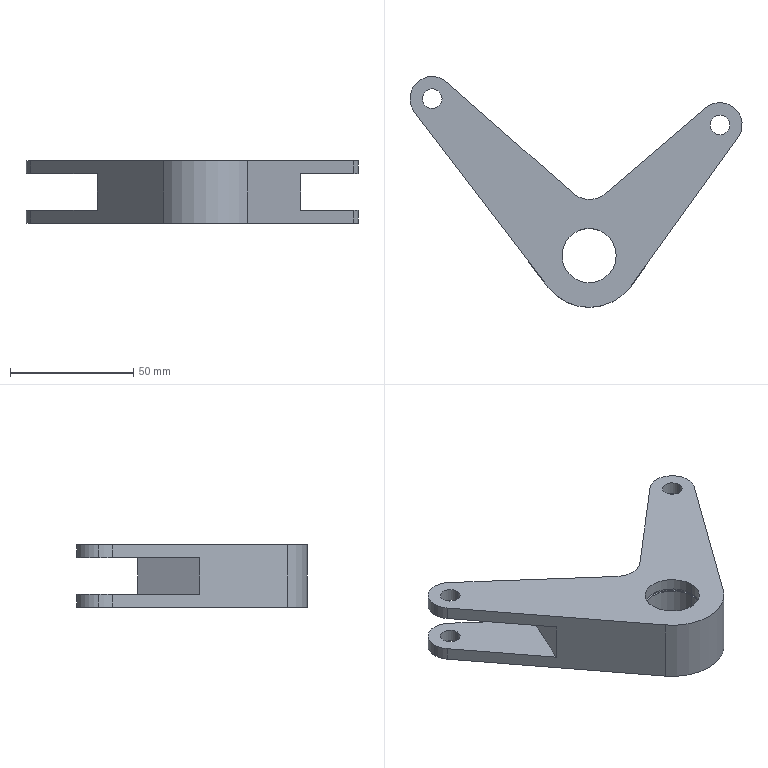Part | SolidWorks | features ICE 6, Extrusion 1, Fillet 1 | 1 solid | 42 faces | box 134.673 x 93.64 x 25.4 mm | volume 86753 mm3 | cylinder 26 | plane 16 | commonest cylinder face diameters 8 x8 18 x6 22 x6 23.3 x4 20 x1 42 x1
STEP:
#1=CARTESIAN_POINT('',(-11.65,0.,-8.1));
#2=VERTEX_POINT('',#1);
#3=CARTESIAN_POINT('',(11.65,0.,-8.1));
#4=VERTEX_POINT('',#3);
#5=CARTESIAN_POINT('',(0.,0.,-8.1));
#6=DIRECTION('',(0.,0.,1.));
#7=DIRECTION('',(1.,0.,0.));
#8=AXIS2_PLACEMENT_3D('',#5,#6,#7);
#9=CIRCLE('',#8,11.65);
#10=EDGE_CURVE('',#2,#4,#9,.T.);
#11=ORIENTED_EDGE('',*,*,#10,.F.);
#12=CARTESIAN_POINT('',(-11.65,0.,-7.));
#13=VERTEX_POINT('',#12);
#14=CARTESIAN_POINT('',(-11.65,0.,-8.1));
#15=DIRECTION('',(0.,0.,1.));
#16=VECTOR('',#15,1000.);
#17=LINE('',#14,#16);
#18=EDGE_CURVE('',#2,#13,#17,.T.);
#19=ORIENTED_EDGE('',*,*,#18,.T.);
#20=CARTESIAN_POINT('',(11.65,0.,-7.));
#21=VERTEX_POINT('',#20);
#22=CARTESIAN_POINT('',(0.,0.,-7.));
#23=DIRECTION('',(0.,0.,1.));
#24=DIRECTION('',(1.,0.,0.));
#25=AXIS2_PLACEMENT_3D('',#22,#23,#24);
#26=CIRCLE('',#25,11.65);
#27=EDGE_CURVE('',#13,#21,#26,.T.);
#28=ORIENTED_EDGE('',*,*,#27,.T.);
#29=CARTESIAN_POINT('',(11.65,0.,-8.1));
#30=DIRECTION('',(0.,0.,1.));
#31=VECTOR('',#30,1000.);
#32=LINE('',#29,#31);
#33=EDGE_CURVE('',#4,#21,#32,.T.);
#34=ORIENTED_EDGE('',*,*,#33,.F.);
#35=EDGE_LOOP('',(#11,#19,#28,#34));
#36=FACE_OUTER_BOUND('',#35,.T.);
#37=CARTESIAN_POINT('',(0.,0.,-8.1));
#38=DIRECTION('',(0.,0.,1.));
#39=DIRECTION('',(1.,0.,0.));
#40=AXIS2_PLACEMENT_3D('',#37,#38,#39);
#41=CYLINDRICAL_SURFACE('',#40,11.65);
#42=ADVANCED_FACE('',(#36),#41,.F.);
#43=CARTESIAN_POINT('',(-11.65,0.,8.1));
#44=VERTEX_POINT('',#43);
#45=CARTESIAN_POINT('',(11.65,0.,8.1));
#46=VERTEX_POINT('',#45);
#47=CARTESIAN_POINT('',(0.,0.,8.1));
#48=DIRECTION('',(0.,0.,1.));
#49=DIRECTION('',(1.,0.,0.));
#50=AXIS2_PLACEMENT_3D('',#47,#48,#49);
#51=CIRCLE('',#50,11.65);
#52=EDGE_CURVE('',#44,#46,#51,.T.);
#53=ORIENTED_EDGE('',*,*,#52,.T.);
#54=CARTESIAN_POINT('',(11.65,0.,7.));
#55=VERTEX_POINT('',#54);
#56=CARTESIAN_POINT('',(11.65,0.,8.1));
#57=DIRECTION('',(0.,0.,-1.));
#58=VECTOR('',#57,1000.);
#59=LINE('',#56,#58);
#60=EDGE_CURVE('',#46,#55,#59,.T.);
#61=ORIENTED_EDGE('',*,*,#60,.T.);
#62=CARTESIAN_POINT('',(-11.65,0.,7.));
#63=VERTEX_POINT('',#62);
#64=CARTESIAN_POINT('',(0.,0.,7.));
#65=DIRECTION('',(0.,0.,1.));
#66=DIRECTION('',(1.,0.,0.));
#67=AXIS2_PLACEMENT_3D('',#64,#65,#66);
#68=CIRCLE('',#67,11.65);
#69=EDGE_CURVE('',#63,#55,#68,.T.);
#70=ORIENTED_EDGE('',*,*,#69,.F.);
#71=CARTESIAN_POINT('',(-11.65,0.,8.1));
#72=DIRECTION('',(0.,0.,-1.));
#73=VECTOR('',#72,1000.);
#74=LINE('',#71,#73);
#75=EDGE_CURVE('',#44,#63,#74,.T.);
#76=ORIENTED_EDGE('',*,*,#75,.F.);
#77=EDGE_LOOP('',(#53,#61,#70,#76));
#78=FACE_OUTER_BOUND('',#77,.T.);
#79=CARTESIAN_POINT('',(0.,0.,8.1));
#80=DIRECTION('',(0.,0.,-1.));
#81=DIRECTION('',(-1.,0.,0.));
#82=AXIS2_PLACEMENT_3D('',#79,#80,#81);
#83=CYLINDRICAL_SURFACE('',#82,11.65);
#84=ADVANCED_FACE('',(#78),#83,.F.);
#85=CARTESIAN_POINT('',(-72.64,63.64,12.7));
#86=VERTEX_POINT('',#85);
#87=CARTESIAN_POINT('',(-70.795,58.181,12.7));
#88=VERTEX_POINT('',#87);
#89=CARTESIAN_POINT('',(-63.64,63.64,12.7));
#90=DIRECTION('',(0.,0.,1.));
#91=DIRECTION('',(1.,0.,0.));
#92=AXIS2_PLACEMENT_3D('',#89,#90,#91);
#93=CIRCLE('',#92,9.);
#94=EDGE_CURVE('',#86,#88,#93,.T.);
#95=ORIENTED_EDGE('',*,*,#94,.F.);
#96=CARTESIAN_POINT('',(-72.64,63.64,7.5));
#97=VERTEX_POINT('',#96);
#98=CARTESIAN_POINT('',(-72.64,63.64,12.7));
#99=DIRECTION('',(0.,0.,-1.));
#100=VECTOR('',#99,1000.);
#101=LINE('',#98,#100);
#102=EDGE_CURVE('',#86,#97,#101,.T.);
#103=ORIENTED_EDGE('',*,*,#102,.T.);
#104=CARTESIAN_POINT('',(-70.795,58.181,7.5));
#105=VERTEX_POINT('',#104);
#106=CARTESIAN_POINT('',(-63.64,63.64,7.5));
#107=DIRECTION('',(0.,0.,1.));
#108=DIRECTION('',(1.,0.,0.));
#109=AXIS2_PLACEMENT_3D('',#106,#107,#108);
#110=CIRCLE('',#109,9.);
#111=EDGE_CURVE('',#97,#105,#110,.T.);
#112=ORIENTED_EDGE('',*,*,#111,.T.);
#113=CARTESIAN_POINT('',(-70.795,58.181,12.7));
#114=DIRECTION('',(0.,0.,-1.));
#115=VECTOR('',#114,1000.);
#116=LINE('',#113,#115);
#117=EDGE_CURVE('',#88,#105,#116,.T.);
#118=ORIENTED_EDGE('',*,*,#117,.F.);
#119=EDGE_LOOP('',(#95,#103,#112,#118));
#120=FACE_OUTER_BOUND('',#119,.T.);
#121=CARTESIAN_POINT('',(-63.64,63.64,12.7));
#122=DIRECTION('',(0.,0.,-1.));
#123=DIRECTION('',(-1.,0.,0.));
#124=AXIS2_PLACEMENT_3D('',#121,#122,#123);
#125=CYLINDRICAL_SURFACE('',#124,9.);
#126=ADVANCED_FACE('',(#120),#125,.T.);
#127=CARTESIAN_POINT('',(49.033,53.033,12.7));
#128=VERTEX_POINT('',#127);
#129=CARTESIAN_POINT('',(57.033,53.033,12.7));
#130=VERTEX_POINT('',#129);
#131=CARTESIAN_POINT('',(53.033,53.033,12.7));
#132=DIRECTION('',(0.,0.,1.));
#133=DIRECTION('',(1.,0.,0.));
#134=AXIS2_PLACEMENT_3D('',#131,#132,#133);
#135=CIRCLE('',#134,4.);
#136=EDGE_CURVE('',#128,#130,#135,.T.);
#137=ORIENTED_EDGE('',*,*,#136,.T.);
#138=CARTESIAN_POINT('',(57.033,53.033,7.5));
#139=VERTEX_POINT('',#138);
#140=CARTESIAN_POINT('',(57.033,53.033,12.7));
#141=DIRECTION('',(0.,0.,-1.));
#142=VECTOR('',#141,1000.);
#143=LINE('',#140,#142);
#144=EDGE_CURVE('',#130,#139,#143,.T.);
#145=ORIENTED_EDGE('',*,*,#144,.T.);
#146=CARTESIAN_POINT('',(49.033,53.033,7.5));
#147=VERTEX_POINT('',#146);
#148=CARTESIAN_POINT('',(53.033,53.033,7.5));
#149=DIRECTION('',(0.,0.,1.));
#150=DIRECTION('',(1.,0.,0.));
#151=AXIS2_PLACEMENT_3D('',#148,#149,#150);
#152=CIRCLE('',#151,4.);
#153=EDGE_CURVE('',#147,#139,#152,.T.);
#154=ORIENTED_EDGE('',*,*,#153,.F.);
#155=CARTESIAN_POINT('',(49.033,53.033,12.7));
#156=DIRECTION('',(0.,0.,-1.));
#157=VECTOR('',#156,1000.);
#158=LINE('',#155,#157);
#159=EDGE_CURVE('',#128,#147,#158,.T.);
#160=ORIENTED_EDGE('',*,*,#159,.F.);
#161=EDGE_LOOP('',(#137,#145,#154,#160));
#162=FACE_OUTER_BOUND('',#161,.T.);
#163=CARTESIAN_POINT('',(53.033,53.033,12.7));
#164=DIRECTION('',(0.,0.,-1.));
#165=DIRECTION('',(-1.,0.,0.));
#166=AXIS2_PLACEMENT_3D('',#163,#164,#165);
#167=CYLINDRICAL_SURFACE('',#166,4.);
#168=ADVANCED_FACE('',(#162),#167,.F.);
#169=CARTESIAN_POINT('',(-67.64,63.64,12.7));
#170=VERTEX_POINT('',#169);
#171=CARTESIAN_POINT('',(-59.64,63.64,12.7));
#172=VERTEX_POINT('',#171);
#173=CARTESIAN_POINT('',(-63.64,63.64,12.7));
#174=DIRECTION('',(0.,0.,1.));
#175=DIRECTION('',(1.,0.,0.));
#176=AXIS2_PLACEMENT_3D('',#173,#174,#175);
#177=CIRCLE('',#176,4.);
#178=EDGE_CURVE('',#170,#172,#177,.T.);
#179=ORIENTED_EDGE('',*,*,#178,.T.);
#180=CARTESIAN_POINT('',(-59.64,63.64,7.5));
#181=VERTEX_POINT('',#180);
#182=CARTESIAN_POINT('',(-59.64,63.64,12.7));
#183=DIRECTION('',(0.,0.,-1.));
#184=VECTOR('',#183,1000.);
#185=LINE('',#182,#184);
#186=EDGE_CURVE('',#172,#181,#185,.T.);
#187=ORIENTED_EDGE('',*,*,#186,.T.);
#188=CARTESIAN_POINT('',(-67.64,63.64,7.5));
#189=VERTEX_POINT('',#188);
#190=CARTESIAN_POINT('',(-63.64,63.64,7.5));
#191=DIRECTION('',(0.,0.,1.));
#192=DIRECTION('',(1.,0.,0.));
#193=AXIS2_PLACEMENT_3D('',#190,#191,#192);
#194=CIRCLE('',#193,4.);
#195=EDGE_CURVE('',#189,#181,#194,.T.);
#196=ORIENTED_EDGE('',*,*,#195,.F.);
#197=CARTESIAN_POINT('',(-67.64,63.64,12.7));
#198=DIRECTION('',(0.,0.,-1.));
#199=VECTOR('',#198,1000.);
#200=LINE('',#197,#199);
#201=EDGE_CURVE('',#170,#189,#200,.T.);
#202=ORIENTED_EDGE('',*,*,#201,.F.);
#203=EDGE_LOOP('',(#179,#187,#196,#202));
#204=FACE_OUTER_BOUND('',#203,.T.);
#205=CARTESIAN_POINT('',(-63.64,63.64,12.7));
#206=DIRECTION('',(0.,0.,-1.));
#207=DIRECTION('',(-1.,0.,0.));
#208=AXIS2_PLACEMENT_3D('',#205,#206,#207);
#209=CYLINDRICAL_SURFACE('',#208,4.);
#210=ADVANCED_FACE('',(#204),#209,.F.);
#211=CARTESIAN_POINT('',(-11.,0.,12.7));
#212=VERTEX_POINT('',#211);
#213=CARTESIAN_POINT('',(11.,0.,12.7));
#214=VERTEX_POINT('',#213);
#215=CARTESIAN_POINT('',(0.,0.,12.7));
#216=DIRECTION('',(0.,0.,1.));
#217=DIRECTION('',(1.,0.,0.));
#218=AXIS2_PLACEMENT_3D('',#215,#216,#217);
#219=CIRCLE('',#218,11.);
#220=EDGE_CURVE('',#212,#214,#219,.T.);
#221=ORIENTED_EDGE('',*,*,#220,.T.);
#222=CARTESIAN_POINT('',(11.,0.,8.1));
#223=VERTEX_POINT('',#222);
#224=CARTESIAN_POINT('',(11.,0.,12.7));
#225=DIRECTION('',(0.,0.,-1.));
#226=VECTOR('',#225,1000.);
#227=LINE('',#224,#226);
#228=EDGE_CURVE('',#214,#223,#227,.T.);
#229=ORIENTED_EDGE('',*,*,#228,.T.);
#230=CARTESIAN_POINT('',(-11.,0.,8.1));
#231=VERTEX_POINT('',#230);
#232=CARTESIAN_POINT('',(0.,0.,8.1));
#233=DIRECTION('',(0.,0.,1.));
#234=DIRECTION('',(1.,0.,0.));
#235=AXIS2_PLACEMENT_3D('',#232,#233,#234);
#236=CIRCLE('',#235,11.);
#237=EDGE_CURVE('',#231,#223,#236,.T.);
#238=ORIENTED_EDGE('',*,*,#237,.F.);
#239=CARTESIAN_POINT('',(-11.,0.,12.7));
#240=DIRECTION('',(0.,0.,-1.));
#241=VECTOR('',#240,1000.);
#242=LINE('',#239,#241);
#243=EDGE_CURVE('',#212,#231,#242,.T.);
#244=ORIENTED_EDGE('',*,*,#243,.F.);
#245=EDGE_LOOP('',(#221,#229,#238,#244));
#246=FACE_OUTER_BOUND('',#245,.T.);
#247=CARTESIAN_POINT('',(0.,0.,12.7));
#248=DIRECTION('',(0.,0.,-1.));
#249=DIRECTION('',(-1.,0.,0.));
#250=AXIS2_PLACEMENT_3D('',#247,#248,#249);
#251=CYLINDRICAL_SURFACE('',#250,11.);
#252=ADVANCED_FACE('',(#246),#251,.F.);
#253=CARTESIAN_POINT('',(49.033,53.033,-7.5));
#254=VERTEX_POINT('',#253);
#255=CARTESIAN_POINT('',(57.033,53.033,-7.5));
#256=VERTEX_POINT('',#255);
#257=CARTESIAN_POINT('',(53.033,53.033,-7.5));
#258=DIRECTION('',(0.,0.,1.));
#259=DIRECTION('',(1.,0.,0.));
#260=AXIS2_PLACEMENT_3D('',#257,#258,#259);
#261=CIRCLE('',#260,4.);
#262=EDGE_CURVE('',#254,#256,#261,.T.);
#263=ORIENTED_EDGE('',*,*,#262,.T.);
#264=CARTESIAN_POINT('',(57.033,53.033,-12.7));
#265=VERTEX_POINT('',#264);
#266=CARTESIAN_POINT('',(57.033,53.033,12.7));
#267=DIRECTION('',(0.,0.,-1.));
#268=VECTOR('',#267,1000.);
#269=LINE('',#266,#268);
#270=EDGE_CURVE('',#256,#265,#269,.T.);
#271=ORIENTED_EDGE('',*,*,#270,.T.);
#272=CARTESIAN_POINT('',(49.033,53.033,-12.7));
#273=VERTEX_POINT('',#272);
#274=CARTESIAN_POINT('',(53.033,53.033,-12.7));
#275=DIRECTION('',(0.,0.,1.));
#276=DIRECTION('',(1.,0.,0.));
#277=AXIS2_PLACEMENT_3D('',#274,#275,#276);
#278=CIRCLE('',#277,4.);
#279=EDGE_CURVE('',#273,#265,#278,.T.);
#280=ORIENTED_EDGE('',*,*,#279,.F.);
#281=CARTESIAN_POINT('',(49.033,53.033,12.7));
#282=DIRECTION('',(0.,0.,-1.));
#283=VECTOR('',#282,1000.);
#284=LINE('',#281,#283);
#285=EDGE_CURVE('',#254,#273,#284,.T.);
#286=ORIENTED_EDGE('',*,*,#285,.F.);
#287=EDGE_LOOP('',(#263,#271,#280,#286));
#288=FACE_OUTER_BOUND('',#287,.T.);
#289=CARTESIAN_POINT('',(53.033,53.033,12.7));
#290=DIRECTION('',(0.,0.,-1.));
#291=DIRECTION('',(-1.,0.,0.));
#292=AXIS2_PLACEMENT_3D('',#289,#290,#291);
#293=CYLINDRICAL_SURFACE('',#292,4.);
#294=ADVANCED_FACE('',(#288),#293,.F.);
#295=CARTESIAN_POINT('',(-67.64,63.64,-7.5));
#296=VERTEX_POINT('',#295);
#297=CARTESIAN_POINT('',(-59.64,63.64,-7.5));
#298=VERTEX_POINT('',#297);
#299=CARTESIAN_POINT('',(-63.64,63.64,-7.5));
#300=DIRECTION('',(0.,0.,1.));
#301=DIRECTION('',(1.,0.,0.));
#302=AXIS2_PLACEMENT_3D('',#299,#300,#301);
#303=CIRCLE('',#302,4.);
#304=EDGE_CURVE('',#296,#298,#303,.T.);
#305=ORIENTED_EDGE('',*,*,#304,.T.);
#306=CARTESIAN_POINT('',(-59.64,63.64,-12.7));
#307=VERTEX_POINT('',#306);
#308=CARTESIAN_POINT('',(-59.64,63.64,12.7));
#309=DIRECTION('',(0.,0.,-1.));
#310=VECTOR('',#309,1000.);
#311=LINE('',#308,#310);
#312=EDGE_CURVE('',#298,#307,#311,.T.);
#313=ORIENTED_EDGE('',*,*,#312,.T.);
#314=CARTESIAN_POINT('',(-67.64,63.64,-12.7));
#315=VERTEX_POINT('',#314);
#316=CARTESIAN_POINT('',(-63.64,63.64,-12.7));
#317=DIRECTION('',(0.,0.,1.));
#318=DIRECTION('',(1.,0.,0.));
#319=AXIS2_PLACEMENT_3D('',#316,#317,#318);
#320=CIRCLE('',#319,4.);
#321=EDGE_CURVE('',#315,#307,#320,.T.);
#322=ORIENTED_EDGE('',*,*,#321,.F.);
#323=CARTESIAN_POINT('',(-67.64,63.64,12.7));
#324=DIRECTION('',(0.,0.,-1.));
#325=VECTOR('',#324,1000.);
#326=LINE('',#323,#325);
#327=EDGE_CURVE('',#296,#315,#326,.T.);
#328=ORIENTED_EDGE('',*,*,#327,.F.);
#329=EDGE_LOOP('',(#305,#313,#322,#328));
#330=FACE_OUTER_BOUND('',#329,.T.);
#331=CARTESIAN_POINT('',(-63.64,63.64,12.7));
#332=DIRECTION('',(0.,0.,-1.));
#333=DIRECTION('',(-1.,0.,0.));
#334=AXIS2_PLACEMENT_3D('',#331,#332,#333);
#335=CYLINDRICAL_SURFACE('',#334,4.);
#336=ADVANCED_FACE('',(#330),#335,.F.);
#337=CARTESIAN_POINT('',(-72.64,63.64,-7.5));
#338=VERTEX_POINT('',#337);
#339=CARTESIAN_POINT('',(-70.795,58.181,-7.5));
#340=VERTEX_POINT('',#339);
#341=CARTESIAN_POINT('',(-63.64,63.64,-7.5));
#342=DIRECTION('',(0.,0.,1.));
#343=DIRECTION('',(1.,0.,0.));
#344=AXIS2_PLACEMENT_3D('',#341,#342,#343);
#345=CIRCLE('',#344,9.);
#346=EDGE_CURVE('',#338,#340,#345,.T.);
#347=ORIENTED_EDGE('',*,*,#346,.F.);
#348=CARTESIAN_POINT('',(-72.64,63.64,-12.7));
#349=VERTEX_POINT('',#348);
#350=CARTESIAN_POINT('',(-72.64,63.64,12.7));
#351=DIRECTION('',(0.,0.,-1.));
#352=VECTOR('',#351,1000.);
#353=LINE('',#350,#352);
#354=EDGE_CURVE('',#338,#349,#353,.T.);
#355=ORIENTED_EDGE('',*,*,#354,.T.);
#356=CARTESIAN_POINT('',(-70.795,58.181,-12.7));
#357=VERTEX_POINT('',#356);
#358=CARTESIAN_POINT('',(-63.64,63.64,-12.7));
#359=DIRECTION('',(0.,0.,1.));
#360=DIRECTION('',(1.,0.,0.));
#361=AXIS2_PLACEMENT_3D('',#358,#359,#360);
#362=CIRCLE('',#361,9.);
#363=EDGE_CURVE('',#349,#357,#362,.T.);
#364=ORIENTED_EDGE('',*,*,#363,.T.);
#365=CARTESIAN_POINT('',(-70.795,58.181,12.7));
#366=DIRECTION('',(0.,0.,-1.));
#367=VECTOR('',#366,1000.);
#368=LINE('',#365,#367);
#369=EDGE_CURVE('',#340,#357,#368,.T.);
#370=ORIENTED_EDGE('',*,*,#369,.F.);
#371=EDGE_LOOP('',(#347,#355,#364,#370));
#372=FACE_OUTER_BOUND('',#371,.T.);
#373=CARTESIAN_POINT('',(-63.64,63.64,12.7));
#374=DIRECTION('',(0.,0.,-1.));
#375=DIRECTION('',(-1.,0.,0.));
#376=AXIS2_PLACEMENT_3D('',#373,#374,#375);
#377=CYLINDRICAL_SURFACE('',#376,9.);
#378=ADVANCED_FACE('',(#372),#377,.T.);
#379=CARTESIAN_POINT('',(-11.,0.,7.));
#380=VERTEX_POINT('',#379);
#381=CARTESIAN_POINT('',(11.,0.,7.));
#382=VERTEX_POINT('',#381);
#383=CARTESIAN_POINT('',(0.,0.,7.));
#384=DIRECTION('',(0.,0.,1.));
#385=DIRECTION('',(1.,0.,0.));
#386=AXIS2_PLACEMENT_3D('',#383,#384,#385);
#387=CIRCLE('',#386,11.);
#388=EDGE_CURVE('',#380,#382,#387,.T.);
#389=ORIENTED_EDGE('',*,*,#388,.T.);
#390=CARTESIAN_POINT('',(11.,0.,-7.));
#391=VERTEX_POINT('',#390);
#392=CARTESIAN_POINT('',(11.,0.,12.7));
#393=DIRECTION('',(0.,0.,-1.));
#394=VECTOR('',#393,1000.);
#395=LINE('',#392,#394);
#396=EDGE_CURVE('',#382,#391,#395,.T.);
#397=ORIENTED_EDGE('',*,*,#396,.T.);
#398=CARTESIAN_POINT('',(-11.,0.,-7.));
#399=VERTEX_POINT('',#398);
#400=CARTESIAN_POINT('',(0.,0.,-7.));
#401=DIRECTION('',(0.,0.,1.));
#402=DIRECTION('',(1.,0.,0.));
#403=AXIS2_PLACEMENT_3D('',#400,#401,#402);
#404=CIRCLE('',#403,11.);
#405=EDGE_CURVE('',#399,#391,#404,.T.);
#406=ORIENTED_EDGE('',*,*,#405,.F.);
#407=CARTESIAN_POINT('',(-11.,0.,12.7));
#408=DIRECTION('',(0.,0.,-1.));
#409=VECTOR('',#408,1000.);
#410=LINE('',#407,#409);
#411=EDGE_CURVE('',#380,#399,#410,.T.);
#412=ORIENTED_EDGE('',*,*,#411,.F.);
#413=EDGE_LOOP('',(#389,#397,#406,#412));
#414=FACE_OUTER_BOUND('',#413,.T.);
#415=CARTESIAN_POINT('',(0.,0.,12.7));
#416=DIRECTION('',(0.,0.,-1.));
#417=DIRECTION('',(-1.,0.,0.));
#418=AXIS2_PLACEMENT_3D('',#415,#416,#417);
#419=CYLINDRICAL_SURFACE('',#418,11.);
#420=ADVANCED_FACE('',(#414),#419,.F.);
#421=CARTESIAN_POINT('',(-11.,0.,-8.1));
#422=VERTEX_POINT('',#421);
#423=CARTESIAN_POINT('',(11.,0.,-8.1));
#424=VERTEX_POINT('',#423);
#425=CARTESIAN_POINT('',(0.,0.,-8.1));
#426=DIRECTION('',(0.,0.,1.));
#427=DIRECTION('',(1.,0.,0.));
#428=AXIS2_PLACEMENT_3D('',#425,#426,#427);
#429=CIRCLE('',#428,11.);
#430=EDGE_CURVE('',#422,#424,#429,.T.);
#431=ORIENTED_EDGE('',*,*,#430,.T.);
#432=CARTESIAN_POINT('',(11.,0.,-12.7));
#433=VERTEX_POINT('',#432);
#434=CARTESIAN_POINT('',(11.,0.,12.7));
#435=DIRECTION('',(0.,0.,-1.));
#436=VECTOR('',#435,1000.);
#437=LINE('',#434,#436);
#438=EDGE_CURVE('',#424,#433,#437,.T.);
#439=ORIENTED_EDGE('',*,*,#438,.T.);
#440=CARTESIAN_POINT('',(-11.,0.,-12.7));
#441=VERTEX_POINT('',#440);
#442=CARTESIAN_POINT('',(0.,0.,-12.7));
#443=DIRECTION('',(0.,0.,1.));
#444=DIRECTION('',(1.,0.,0.));
#445=AXIS2_PLACEMENT_3D('',#442,#443,#444);
#446=CIRCLE('',#445,11.);
#447=EDGE_CURVE('',#441,#433,#446,.T.);
#448=ORIENTED_EDGE('',*,*,#447,.F.);
#449=CARTESIAN_POINT('',(-11.,0.,12.7));
#450=DIRECTION('',(0.,0.,-1.));
#451=VECTOR('',#450,1000.);
#452=LINE('',#449,#451);
#453=EDGE_CURVE('',#422,#441,#452,.T.);
#454=ORIENTED_EDGE('',*,*,#453,.F.);
#455=EDGE_LOOP('',(#431,#439,#448,#454));
#456=FACE_OUTER_BOUND('',#455,.T.);
#457=CARTESIAN_POINT('',(0.,0.,12.7));
#458=DIRECTION('',(0.,0.,-1.));
#459=DIRECTION('',(-1.,0.,0.));
#460=AXIS2_PLACEMENT_3D('',#457,#458,#459);
#461=CYLINDRICAL_SURFACE('',#460,11.);
#462=ADVANCED_FACE('',(#456),#461,.F.);
#463=ORIENTED_EDGE('',*,*,#153,.T.);
#464=CARTESIAN_POINT('',(53.033,53.033,7.5));
#465=DIRECTION('',(0.,0.,1.));
#466=DIRECTION('',(1.,0.,0.));
#467=AXIS2_PLACEMENT_3D('',#464,#465,#466);
#468=CIRCLE('',#467,4.);
#469=EDGE_CURVE('',#139,#147,#468,.T.);
#470=ORIENTED_EDGE('',*,*,#469,.T.);
#471=EDGE_LOOP('',(#463,#470));
#472=FACE_BOUND('',#471,.T.);
#473=CARTESIAN_POINT('',(26.892,42.51,7.5));
#474=VERTEX_POINT('',#473);
#475=CARTESIAN_POINT('',(38.684,17.744,7.5));
#476=VERTEX_POINT('',#475);
#477=CARTESIAN_POINT('',(27.638,40.942,7.5));
#478=DIRECTION('',(0.4299,-0.9029,0.));
#479=VECTOR('',#478,1000.);
#480=LINE('',#477,#479);
#481=EDGE_CURVE('',#474,#476,#480,.T.);
#482=ORIENTED_EDGE('',*,*,#481,.F.);
#483=CARTESIAN_POINT('',(47.182,59.871,7.5));
#484=VERTEX_POINT('',#483);
#485=CARTESIAN_POINT('',(47.182,59.871,7.5));
#486=DIRECTION('',(-0.7598,-0.6501,0.));
#487=VECTOR('',#486,1000.);
#488=LINE('',#485,#487);
#489=EDGE_CURVE('',#484,#474,#488,.T.);
#490=ORIENTED_EDGE('',*,*,#489,.F.);
#491=CARTESIAN_POINT('',(60.333,47.769,7.5));
#492=VERTEX_POINT('',#491);
#493=CARTESIAN_POINT('',(53.033,53.033,7.5));
#494=DIRECTION('',(0.,0.,1.));
#495=DIRECTION('',(1.,0.,0.));
#496=AXIS2_PLACEMENT_3D('',#493,#494,#495);
#497=CIRCLE('',#496,9.);
#498=EDGE_CURVE('',#492,#484,#497,.T.);
#499=ORIENTED_EDGE('',*,*,#498,.F.);
#500=CARTESIAN_POINT('',(17.034,-12.282,7.5));
#501=DIRECTION('',(0.5849,0.8111,0.));
#502=VECTOR('',#501,1000.);
#503=LINE('',#500,#502);
#504=EDGE_CURVE('',#476,#492,#503,.T.);
#505=ORIENTED_EDGE('',*,*,#504,.F.);
#506=EDGE_LOOP('',(#482,#490,#499,#505));
#507=FACE_OUTER_BOUND('',#506,.T.);
#508=CARTESIAN_POINT('',(53.033,53.033,7.5));
#509=DIRECTION('',(0.,0.,1.));
#510=DIRECTION('',(1.,0.,0.));
#511=AXIS2_PLACEMENT_3D('',#508,#509,#510);
#512=PLANE('',#511);
#513=ADVANCED_FACE('',(#472,#507),#512,.F.);
#514=ORIENTED_EDGE('',*,*,#304,.F.);
#515=CARTESIAN_POINT('',(-63.64,63.64,-7.5));
#516=DIRECTION('',(0.,0.,1.));
#517=DIRECTION('',(1.,0.,0.));
#518=AXIS2_PLACEMENT_3D('',#515,#516,#517);
#519=CIRCLE('',#518,4.);
#520=EDGE_CURVE('',#298,#296,#519,.T.);
#521=ORIENTED_EDGE('',*,*,#520,.F.);
#522=EDGE_LOOP('',(#514,#521));
#523=FACE_BOUND('',#522,.T.);
#524=CARTESIAN_POINT('',(-43.746,22.722,-7.5));
#525=VERTEX_POINT('',#524);
#526=CARTESIAN_POINT('',(-70.795,58.181,-7.5));
#527=DIRECTION('',(0.6065,-0.7951,0.));
#528=VECTOR('',#527,1000.);
#529=LINE('',#526,#528);
#530=EDGE_CURVE('',#340,#525,#529,.T.);
#531=ORIENTED_EDGE('',*,*,#530,.T.);
#532=CARTESIAN_POINT('',(-32.101,47.818,-7.5));
#533=VERTEX_POINT('',#532);
#534=CARTESIAN_POINT('',(-15.026,84.614,-7.5));
#535=DIRECTION('',(0.4209,0.9071,0.));
#536=VECTOR('',#535,1000.);
#537=LINE('',#534,#536);
#538=EDGE_CURVE('',#525,#533,#537,.T.);
#539=ORIENTED_EDGE('',*,*,#538,.T.);
#540=CARTESIAN_POINT('',(-57.686,70.389,-7.5));
#541=VERTEX_POINT('',#540);
#542=CARTESIAN_POINT('',(-6.515,25.248,-7.5));
#543=DIRECTION('',(-0.7499,0.6615,0.));
#544=VECTOR('',#543,1000.);
#545=LINE('',#542,#544);
#546=EDGE_CURVE('',#533,#541,#545,.T.);
#547=ORIENTED_EDGE('',*,*,#546,.T.);
#548=CARTESIAN_POINT('',(-63.64,63.64,-7.5));
#549=DIRECTION('',(0.,0.,1.));
#550=DIRECTION('',(1.,0.,0.));
#551=AXIS2_PLACEMENT_3D('',#548,#549,#550);
#552=CIRCLE('',#551,9.);
#553=EDGE_CURVE('',#541,#338,#552,.T.);
#554=ORIENTED_EDGE('',*,*,#553,.T.);
#555=ORIENTED_EDGE('',*,*,#346,.T.);
#556=EDGE_LOOP('',(#531,#539,#547,#554,#555));
#557=FACE_OUTER_BOUND('',#556,.T.);
#558=CARTESIAN_POINT('',(53.033,53.033,-7.5));
#559=DIRECTION('',(0.,0.,1.));
#560=DIRECTION('',(1.,0.,0.));
#561=AXIS2_PLACEMENT_3D('',#558,#559,#560);
#562=PLANE('',#561);
#563=ADVANCED_FACE('',(#523,#557),#562,.T.);
#564=CARTESIAN_POINT('',(17.034,-12.282,12.7));
#565=VERTEX_POINT('',#564);
#566=CARTESIAN_POINT('',(17.034,-12.282,-12.7));
#567=VERTEX_POINT('',#566);
#568=CARTESIAN_POINT('',(17.034,-12.282,12.7));
#569=DIRECTION('',(0.,0.,-1.));
#570=VECTOR('',#569,1000.);
#571=LINE('',#568,#570);
#572=EDGE_CURVE('',#565,#567,#571,.T.);
#573=ORIENTED_EDGE('',*,*,#572,.F.);
#574=CARTESIAN_POINT('',(-16.697,-12.737,12.7));
#575=VERTEX_POINT('',#574);
#576=CARTESIAN_POINT('',(0.,0.,12.7));
#577=DIRECTION('',(0.,0.,1.));
#578=DIRECTION('',(1.,0.,0.));
#579=AXIS2_PLACEMENT_3D('',#576,#577,#578);
#580=CIRCLE('',#579,21.);
#581=EDGE_CURVE('',#575,#565,#580,.T.);
#582=ORIENTED_EDGE('',*,*,#581,.F.);
#583=CARTESIAN_POINT('',(-16.697,-12.737,-12.7));
#584=VERTEX_POINT('',#583);
#585=CARTESIAN_POINT('',(-16.697,-12.737,12.7));
#586=DIRECTION('',(0.,0.,-1.));
#587=VECTOR('',#586,1000.);
#588=LINE('',#585,#587);
#589=EDGE_CURVE('',#575,#584,#588,.T.);
#590=ORIENTED_EDGE('',*,*,#589,.T.);
#591=CARTESIAN_POINT('',(0.,0.,-12.7));
#592=DIRECTION('',(0.,0.,1.));
#593=DIRECTION('',(1.,0.,0.));
#594=AXIS2_PLACEMENT_3D('',#591,#592,#593);
#595=CIRCLE('',#594,21.);
#596=EDGE_CURVE('',#584,#567,#595,.T.);
#597=ORIENTED_EDGE('',*,*,#596,.T.);
#598=EDGE_LOOP('',(#573,#582,#590,#597));
#599=FACE_OUTER_BOUND('',#598,.T.);
#600=CARTESIAN_POINT('',(0.,0.,12.7));
#601=DIRECTION('',(0.,0.,-1.));
#602=DIRECTION('',(-1.,0.,0.));
#603=AXIS2_PLACEMENT_3D('',#600,#601,#602);
#604=CYLINDRICAL_SURFACE('',#603,21.);
#605=ADVANCED_FACE('',(#599),#604,.T.);
#606=ORIENTED_EDGE('',*,*,#262,.F.);
#607=CARTESIAN_POINT('',(53.033,53.033,-7.5));
#608=DIRECTION('',(0.,0.,1.));
#609=DIRECTION('',(1.,0.,0.));
#610=AXIS2_PLACEMENT_3D('',#607,#608,#609);
#611=CIRCLE('',#610,4.);
#612=EDGE_CURVE('',#256,#254,#611,.T.);
#613=ORIENTED_EDGE('',*,*,#612,.F.);
#614=EDGE_LOOP('',(#606,#613));
#615=FACE_BOUND('',#614,.T.);
#616=CARTESIAN_POINT('',(47.182,59.871,-7.5));
#617=VERTEX_POINT('',#616);
#618=CARTESIAN_POINT('',(26.892,42.51,-7.5));
#619=VERTEX_POINT('',#618);
#620=CARTESIAN_POINT('',(47.182,59.871,-7.5));
#621=DIRECTION('',(-0.7598,-0.6501,0.));
#622=VECTOR('',#621,1000.);
#623=LINE('',#620,#622);
#624=EDGE_CURVE('',#617,#619,#623,.T.);
#625=ORIENTED_EDGE('',*,*,#624,.T.);
#626=CARTESIAN_POINT('',(38.684,17.744,-7.5));
#627=VERTEX_POINT('',#626);
#628=CARTESIAN_POINT('',(27.638,40.942,-7.5));
#629=DIRECTION('',(0.4299,-0.9029,0.));
#630=VECTOR('',#629,1000.);
#631=LINE('',#628,#630);
#632=EDGE_CURVE('',#619,#627,#631,.T.);
#633=ORIENTED_EDGE('',*,*,#632,.T.);
#634=CARTESIAN_POINT('',(60.333,47.769,-7.5));
#635=VERTEX_POINT('',#634);
#636=CARTESIAN_POINT('',(17.034,-12.282,-7.5));
#637=DIRECTION('',(0.5849,0.8111,0.));
#638=VECTOR('',#637,1000.);
#639=LINE('',#636,#638);
#640=EDGE_CURVE('',#627,#635,#639,.T.);
#641=ORIENTED_EDGE('',*,*,#640,.T.);
#642=CARTESIAN_POINT('',(53.033,53.033,-7.5));
#643=DIRECTION('',(0.,0.,1.));
#644=DIRECTION('',(1.,0.,0.));
#645=AXIS2_PLACEMENT_3D('',#642,#643,#644);
#646=CIRCLE('',#645,9.);
#647=EDGE_CURVE('',#635,#617,#646,.T.);
#648=ORIENTED_EDGE('',*,*,#647,.T.);
#649=EDGE_LOOP('',(#625,#633,#641,#648));
#650=FACE_OUTER_BOUND('',#649,.T.);
#651=CARTESIAN_POINT('',(53.033,53.033,-7.5));
#652=DIRECTION('',(0.,0.,1.));
#653=DIRECTION('',(1.,0.,0.));
#654=AXIS2_PLACEMENT_3D('',#651,#652,#653);
#655=PLANE('',#654);
#656=ADVANCED_FACE('',(#615,#650),#655,.T.);
#657=ORIENTED_EDGE('',*,*,#195,.T.);
#658=CARTESIAN_POINT('',(-63.64,63.64,7.5));
#659=DIRECTION('',(0.,0.,1.));
#660=DIRECTION('',(1.,0.,0.));
#661=AXIS2_PLACEMENT_3D('',#658,#659,#660);
#662=CIRCLE('',#661,4.);
#663=EDGE_CURVE('',#181,#189,#662,.T.);
#664=ORIENTED_EDGE('',*,*,#663,.T.);
#665=EDGE_LOOP('',(#657,#664));
#666=FACE_BOUND('',#665,.T.);
#667=CARTESIAN_POINT('',(-43.746,22.722,7.5));
#668=VERTEX_POINT('',#667);
#669=CARTESIAN_POINT('',(-32.101,47.818,7.5));
#670=VERTEX_POINT('',#669);
#671=CARTESIAN_POINT('',(-15.026,84.614,7.5));
#672=DIRECTION('',(0.4209,0.9071,0.));
#673=VECTOR('',#672,1000.);
#674=LINE('',#671,#673);
#675=EDGE_CURVE('',#668,#670,#674,.T.);
#676=ORIENTED_EDGE('',*,*,#675,.F.);
#677=CARTESIAN_POINT('',(-70.795,58.181,7.5));
#678=DIRECTION('',(0.6065,-0.7951,0.));
#679=VECTOR('',#678,1000.);
#680=LINE('',#677,#679);
#681=EDGE_CURVE('',#105,#668,#680,.T.);
#682=ORIENTED_EDGE('',*,*,#681,.F.);
#683=ORIENTED_EDGE('',*,*,#111,.F.);
#684=CARTESIAN_POINT('',(-57.686,70.389,7.5));
#685=VERTEX_POINT('',#684);
#686=CARTESIAN_POINT('',(-63.64,63.64,7.5));
#687=DIRECTION('',(0.,0.,1.));
#688=DIRECTION('',(1.,0.,0.));
#689=AXIS2_PLACEMENT_3D('',#686,#687,#688);
#690=CIRCLE('',#689,9.);
#691=EDGE_CURVE('',#685,#97,#690,.T.);
#692=ORIENTED_EDGE('',*,*,#691,.F.);
#693=CARTESIAN_POINT('',(-6.515,25.248,7.5));
#694=DIRECTION('',(-0.7499,0.6615,0.));
#695=VECTOR('',#694,1000.);
#696=LINE('',#693,#695);
#697=EDGE_CURVE('',#670,#685,#696,.T.);
#698=ORIENTED_EDGE('',*,*,#697,.F.);
#699=EDGE_LOOP('',(#676,#682,#683,#692,#698));
#700=FACE_OUTER_BOUND('',#699,.T.);
#701=CARTESIAN_POINT('',(53.033,53.033,7.5));
#702=DIRECTION('',(0.,0.,1.));
#703=DIRECTION('',(1.,0.,0.));
#704=AXIS2_PLACEMENT_3D('',#701,#702,#703);
#705=PLANE('',#704);
#706=ADVANCED_FACE('',(#666,#700),#705,.F.);
#707=ORIENTED_EDGE('',*,*,#438,.F.);
#708=CARTESIAN_POINT('',(0.,0.,-8.1));
#709=DIRECTION('',(0.,0.,1.));
#710=DIRECTION('',(1.,0.,0.));
#711=AXIS2_PLACEMENT_3D('',#708,#709,#710);
#712=CIRCLE('',#711,11.);
#713=EDGE_CURVE('',#424,#422,#712,.T.);
#714=ORIENTED_EDGE('',*,*,#713,.T.);
#715=ORIENTED_EDGE('',*,*,#453,.T.);
#716=CARTESIAN_POINT('',(0.,0.,-12.7));
#717=DIRECTION('',(0.,0.,1.));
#718=DIRECTION('',(1.,0.,0.));
#719=AXIS2_PLACEMENT_3D('',#716,#717,#718);
#720=CIRCLE('',#719,11.);
#721=EDGE_CURVE('',#433,#441,#720,.T.);
#722=ORIENTED_EDGE('',*,*,#721,.F.);
#723=EDGE_LOOP('',(#707,#714,#715,#722));
#724=FACE_OUTER_BOUND('',#723,.T.);
#725=CARTESIAN_POINT('',(0.,0.,12.7));
#726=DIRECTION('',(0.,0.,-1.));
#727=DIRECTION('',(-1.,0.,0.));
#728=AXIS2_PLACEMENT_3D('',#725,#726,#727);
#729=CYLINDRICAL_SURFACE('',#728,11.);
#730=ADVANCED_FACE('',(#724),#729,.F.);
#731=ORIENTED_EDGE('',*,*,#396,.F.);
#732=CARTESIAN_POINT('',(0.,0.,7.));
#733=DIRECTION('',(0.,0.,1.));
#734=DIRECTION('',(1.,0.,0.));
#735=AXIS2_PLACEMENT_3D('',#732,#733,#734);
#736=CIRCLE('',#735,11.);
#737=EDGE_CURVE('',#382,#380,#736,.T.);
#738=ORIENTED_EDGE('',*,*,#737,.T.);
#739=ORIENTED_EDGE('',*,*,#411,.T.);
#740=CARTESIAN_POINT('',(0.,0.,-7.));
#741=DIRECTION('',(0.,0.,1.));
#742=DIRECTION('',(1.,0.,0.));
#743=AXIS2_PLACEMENT_3D('',#740,#741,#742);
#744=CIRCLE('',#743,11.);
#745=EDGE_CURVE('',#391,#399,#744,.T.);
#746=ORIENTED_EDGE('',*,*,#745,.F.);
#747=EDGE_LOOP('',(#731,#738,#739,#746));
#748=FACE_OUTER_BOUND('',#747,.T.);
#749=CARTESIAN_POINT('',(0.,0.,12.7));
#750=DIRECTION('',(0.,0.,-1.));
#751=DIRECTION('',(-1.,0.,0.));
#752=AXIS2_PLACEMENT_3D('',#749,#750,#751);
#753=CYLINDRICAL_SURFACE('',#752,11.);
#754=ADVANCED_FACE('',(#748),#753,.F.);
#755=ORIENTED_EDGE('',*,*,#354,.F.);
#756=ORIENTED_EDGE('',*,*,#553,.F.);
#757=CARTESIAN_POINT('',(-57.686,70.389,-12.7));
#758=VERTEX_POINT('',#757);
#759=CARTESIAN_POINT('',(-57.686,70.389,-12.7));
#760=DIRECTION('',(0.,0.,1.));
#761=VECTOR('',#760,1000.);
#762=LINE('',#759,#761);
#763=EDGE_CURVE('',#758,#541,#762,.T.);
#764=ORIENTED_EDGE('',*,*,#763,.F.);
#765=CARTESIAN_POINT('',(-63.64,63.64,-12.7));
#766=DIRECTION('',(0.,0.,1.));
#767=DIRECTION('',(1.,0.,0.));
#768=AXIS2_PLACEMENT_3D('',#765,#766,#767);
#769=CIRCLE('',#768,9.);
#770=EDGE_CURVE('',#758,#349,#769,.T.);
#771=ORIENTED_EDGE('',*,*,#770,.T.);
#772=EDGE_LOOP('',(#755,#756,#764,#771));
#773=FACE_OUTER_BOUND('',#772,.T.);
#774=CARTESIAN_POINT('',(-63.64,63.64,12.7));
#775=DIRECTION('',(0.,0.,-1.));
#776=DIRECTION('',(-1.,0.,0.));
#777=AXIS2_PLACEMENT_3D('',#774,#775,#776);
#778=CYLINDRICAL_SURFACE('',#777,9.);
#779=ADVANCED_FACE('',(#773),#778,.T.);
#780=CARTESIAN_POINT('',(-43.746,22.722,12.7));
#781=DIRECTION('',(0.,0.,-1.));
#782=VECTOR('',#781,1000.);
#783=LINE('',#780,#782);
#784=EDGE_CURVE('',#668,#525,#783,.T.);
#785=ORIENTED_EDGE('',*,*,#784,.T.);
#786=ORIENTED_EDGE('',*,*,#530,.F.);
#787=ORIENTED_EDGE('',*,*,#369,.T.);
#788=CARTESIAN_POINT('',(-16.697,-12.737,-12.7));
#789=DIRECTION('',(0.6065,-0.7951,0.));
#790=VECTOR('',#789,1000.);
#791=LINE('',#788,#790);
#792=EDGE_CURVE('',#357,#584,#791,.T.);
#793=ORIENTED_EDGE('',*,*,#792,.T.);
#794=ORIENTED_EDGE('',*,*,#589,.F.);
#795=CARTESIAN_POINT('',(-16.697,-12.737,12.7));
#796=DIRECTION('',(0.6065,-0.7951,0.));
#797=VECTOR('',#796,1000.);
#798=LINE('',#795,#797);
#799=EDGE_CURVE('',#88,#575,#798,.T.);
#800=ORIENTED_EDGE('',*,*,#799,.F.);
#801=ORIENTED_EDGE('',*,*,#117,.T.);
#802=ORIENTED_EDGE('',*,*,#681,.T.);
#803=EDGE_LOOP('',(#785,#786,#787,#793,#794,#800,#801,#802));
#804=FACE_OUTER_BOUND('',#803,.T.);
#805=CARTESIAN_POINT('',(-16.697,-12.737,12.7));
#806=DIRECTION('',(0.7951,0.6065,0.));
#807=DIRECTION('',(-0.6065,0.7951,0.));
#808=AXIS2_PLACEMENT_3D('',#805,#806,#807);
#809=PLANE('',#808);
#810=ADVANCED_FACE('',(#804),#809,.F.);
#811=CARTESIAN_POINT('',(38.684,17.744,12.7));
#812=DIRECTION('',(0.,0.,-1.));
#813=VECTOR('',#812,1000.);
#814=LINE('',#811,#813);
#815=EDGE_CURVE('',#476,#627,#814,.T.);
#816=ORIENTED_EDGE('',*,*,#815,.F.);
#817=ORIENTED_EDGE('',*,*,#504,.T.);
#818=CARTESIAN_POINT('',(60.333,47.769,12.7));
#819=VERTEX_POINT('',#818);
#820=CARTESIAN_POINT('',(60.333,47.769,12.7));
#821=DIRECTION('',(0.,0.,-1.));
#822=VECTOR('',#821,1000.);
#823=LINE('',#820,#822);
#824=EDGE_CURVE('',#819,#492,#823,.T.);
#825=ORIENTED_EDGE('',*,*,#824,.F.);
#826=CARTESIAN_POINT('',(17.034,-12.282,12.7));
#827=DIRECTION('',(0.5849,0.8111,0.));
#828=VECTOR('',#827,1000.);
#829=LINE('',#826,#828);
#830=EDGE_CURVE('',#565,#819,#829,.T.);
#831=ORIENTED_EDGE('',*,*,#830,.F.);
#832=ORIENTED_EDGE('',*,*,#572,.T.);
#833=CARTESIAN_POINT('',(60.333,47.769,-12.7));
#834=VERTEX_POINT('',#833);
#835=CARTESIAN_POINT('',(17.034,-12.282,-12.7));
#836=DIRECTION('',(0.5849,0.8111,0.));
#837=VECTOR('',#836,1000.);
#838=LINE('',#835,#837);
#839=EDGE_CURVE('',#567,#834,#838,.T.);
#840=ORIENTED_EDGE('',*,*,#839,.T.);
#841=CARTESIAN_POINT('',(60.333,47.769,12.7));
#842=DIRECTION('',(0.,0.,-1.));
#843=VECTOR('',#842,1000.);
#844=LINE('',#841,#843);
#845=EDGE_CURVE('',#635,#834,#844,.T.);
#846=ORIENTED_EDGE('',*,*,#845,.F.);
#847=ORIENTED_EDGE('',*,*,#640,.F.);
#848=EDGE_LOOP('',(#816,#817,#825,#831,#832,#840,#846,#847));
#849=FACE_OUTER_BOUND('',#848,.T.);
#850=CARTESIAN_POINT('',(17.034,-12.282,12.7));
#851=DIRECTION('',(-0.8111,0.5849,0.));
#852=DIRECTION('',(-0.5849,-0.8111,0.));
#853=AXIS2_PLACEMENT_3D('',#850,#851,#852);
#854=PLANE('',#853);
#855=ADVANCED_FACE('',(#849),#854,.F.);
#856=ORIENTED_EDGE('',*,*,#312,.F.);
#857=ORIENTED_EDGE('',*,*,#520,.T.);
#858=ORIENTED_EDGE('',*,*,#327,.T.);
#859=CARTESIAN_POINT('',(-63.64,63.64,-12.7));
#860=DIRECTION('',(0.,0.,1.));
#861=DIRECTION('',(1.,0.,0.));
#862=AXIS2_PLACEMENT_3D('',#859,#860,#861);
#863=CIRCLE('',#862,4.);
#864=EDGE_CURVE('',#307,#315,#863,.T.);
#865=ORIENTED_EDGE('',*,*,#864,.F.);
#866=EDGE_LOOP('',(#856,#857,#858,#865));
#867=FACE_OUTER_BOUND('',#866,.T.);
#868=CARTESIAN_POINT('',(-63.64,63.64,12.7));
#869=DIRECTION('',(0.,0.,-1.));
#870=DIRECTION('',(-1.,0.,0.));
#871=AXIS2_PLACEMENT_3D('',#868,#869,#870);
#872=CYLINDRICAL_SURFACE('',#871,4.);
#873=ADVANCED_FACE('',(#867),#872,.F.);
#874=ORIENTED_EDGE('',*,*,#270,.F.);
#875=ORIENTED_EDGE('',*,*,#612,.T.);
#876=ORIENTED_EDGE('',*,*,#285,.T.);
#877=CARTESIAN_POINT('',(53.033,53.033,-12.7));
#878=DIRECTION('',(0.,0.,1.));
#879=DIRECTION('',(1.,0.,0.));
#880=AXIS2_PLACEMENT_3D('',#877,#878,#879);
#881=CIRCLE('',#880,4.);
#882=EDGE_CURVE('',#265,#273,#881,.T.);
#883=ORIENTED_EDGE('',*,*,#882,.F.);
#884=EDGE_LOOP('',(#874,#875,#876,#883));
#885=FACE_OUTER_BOUND('',#884,.T.);
#886=CARTESIAN_POINT('',(53.033,53.033,12.7));
#887=DIRECTION('',(0.,0.,-1.));
#888=DIRECTION('',(-1.,0.,0.));
#889=AXIS2_PLACEMENT_3D('',#886,#887,#888);
#890=CYLINDRICAL_SURFACE('',#889,4.);
#891=ADVANCED_FACE('',(#885),#890,.F.);
#892=ORIENTED_EDGE('',*,*,#228,.F.);
#893=CARTESIAN_POINT('',(0.,0.,12.7));
#894=DIRECTION('',(0.,0.,1.));
#895=DIRECTION('',(1.,0.,0.));
#896=AXIS2_PLACEMENT_3D('',#893,#894,#895);
#897=CIRCLE('',#896,11.);
#898=EDGE_CURVE('',#214,#212,#897,.T.);
#899=ORIENTED_EDGE('',*,*,#898,.T.);
#900=ORIENTED_EDGE('',*,*,#243,.T.);
#901=CARTESIAN_POINT('',(0.,0.,8.1));
#902=DIRECTION('',(0.,0.,1.));
#903=DIRECTION('',(1.,0.,0.));
#904=AXIS2_PLACEMENT_3D('',#901,#902,#903);
#905=CIRCLE('',#904,11.);
#906=EDGE_CURVE('',#223,#231,#905,.T.);
#907=ORIENTED_EDGE('',*,*,#906,.F.);
#908=EDGE_LOOP('',(#892,#899,#900,#907));
#909=FACE_OUTER_BOUND('',#908,.T.);
#910=CARTESIAN_POINT('',(0.,0.,12.7));
#911=DIRECTION('',(0.,0.,-1.));
#912=DIRECTION('',(-1.,0.,0.));
#913=AXIS2_PLACEMENT_3D('',#910,#911,#912);
#914=CYLINDRICAL_SURFACE('',#913,11.);
#915=ADVANCED_FACE('',(#909),#914,.F.);
#916=ORIENTED_EDGE('',*,*,#647,.F.);
#917=ORIENTED_EDGE('',*,*,#845,.T.);
#918=CARTESIAN_POINT('',(47.182,59.871,-12.7));
#919=VERTEX_POINT('',#918);
#920=CARTESIAN_POINT('',(53.033,53.033,-12.7));
#921=DIRECTION('',(0.,0.,1.));
#922=DIRECTION('',(1.,0.,0.));
#923=AXIS2_PLACEMENT_3D('',#920,#921,#922);
#924=CIRCLE('',#923,9.);
#925=EDGE_CURVE('',#834,#919,#924,.T.);
#926=ORIENTED_EDGE('',*,*,#925,.T.);
#927=CARTESIAN_POINT('',(47.182,59.871,-12.7));
#928=DIRECTION('',(0.,0.,1.));
#929=VECTOR('',#928,1000.);
#930=LINE('',#927,#929);
#931=EDGE_CURVE('',#919,#617,#930,.T.);
#932=ORIENTED_EDGE('',*,*,#931,.T.);
#933=EDGE_LOOP('',(#916,#917,#926,#932));
#934=FACE_OUTER_BOUND('',#933,.T.);
#935=CARTESIAN_POINT('',(53.033,53.033,12.7));
#936=DIRECTION('',(0.,0.,-1.));
#937=DIRECTION('',(-1.,0.,0.));
#938=AXIS2_PLACEMENT_3D('',#935,#936,#937);
#939=CYLINDRICAL_SURFACE('',#938,9.);
#940=ADVANCED_FACE('',(#934),#939,.T.);
#941=CARTESIAN_POINT('',(6.601,25.149,-12.7));
#942=VERTEX_POINT('',#941);
#943=CARTESIAN_POINT('',(6.601,25.149,12.7));
#944=VERTEX_POINT('',#943);
#945=CARTESIAN_POINT('',(6.601,25.149,-12.7));
#946=DIRECTION('',(0.,0.,1.));
#947=VECTOR('',#946,1000.);
#948=LINE('',#945,#947);
#949=EDGE_CURVE('',#942,#944,#948,.T.);
#950=ORIENTED_EDGE('',*,*,#949,.T.);
#951=CARTESIAN_POINT('',(47.182,59.871,12.7));
#952=VERTEX_POINT('',#951);
#953=CARTESIAN_POINT('',(6.601,25.149,12.7));
#954=DIRECTION('',(0.7598,0.6501,0.));
#955=VECTOR('',#954,1000.);
#956=LINE('',#953,#955);
#957=EDGE_CURVE('',#944,#952,#956,.T.);
#958=ORIENTED_EDGE('',*,*,#957,.T.);
#959=CARTESIAN_POINT('',(47.182,59.871,-12.7));
#960=DIRECTION('',(0.,0.,1.));
#961=VECTOR('',#960,1000.);
#962=LINE('',#959,#961);
#963=EDGE_CURVE('',#484,#952,#962,.T.);
#964=ORIENTED_EDGE('',*,*,#963,.F.);
#965=ORIENTED_EDGE('',*,*,#489,.T.);
#966=CARTESIAN_POINT('',(26.892,42.51,12.7));
#967=DIRECTION('',(0.,0.,-1.));
#968=VECTOR('',#967,1000.);
#969=LINE('',#966,#968);
#970=EDGE_CURVE('',#474,#619,#969,.T.);
#971=ORIENTED_EDGE('',*,*,#970,.T.);
#972=ORIENTED_EDGE('',*,*,#624,.F.);
#973=ORIENTED_EDGE('',*,*,#931,.F.);
#974=CARTESIAN_POINT('',(6.601,25.149,-12.7));
#975=DIRECTION('',(0.7598,0.6501,0.));
#976=VECTOR('',#975,1000.);
#977=LINE('',#974,#976);
#978=EDGE_CURVE('',#942,#919,#977,.T.);
#979=ORIENTED_EDGE('',*,*,#978,.F.);
#980=EDGE_LOOP('',(#950,#958,#964,#965,#971,#972,#973,#979));
#981=FACE_OUTER_BOUND('',#980,.T.);
#982=CARTESIAN_POINT('',(6.601,25.149,-12.7));
#983=DIRECTION('',(0.6501,-0.7598,0.));
#984=DIRECTION('',(0.7598,0.6501,0.));
#985=AXIS2_PLACEMENT_3D('',#982,#983,#984);
#986=PLANE('',#985);
#987=ADVANCED_FACE('',(#981),#986,.F.);
#988=CARTESIAN_POINT('',(-6.515,25.248,-12.7));
#989=VERTEX_POINT('',#988);
#990=CARTESIAN_POINT('',(-6.515,25.248,12.7));
#991=VERTEX_POINT('',#990);
#992=CARTESIAN_POINT('',(-6.515,25.248,-12.7));
#993=DIRECTION('',(0.,0.,1.));
#994=VECTOR('',#993,1000.);
#995=LINE('',#992,#994);
#996=EDGE_CURVE('',#989,#991,#995,.T.);
#997=ORIENTED_EDGE('',*,*,#996,.T.);
#998=CARTESIAN_POINT('',(0.1001,32.747,12.7));
#999=DIRECTION('',(0.,0.,1.));
#1000=DIRECTION('',(1.,0.,0.));
#1001=AXIS2_PLACEMENT_3D('',#998,#999,#1000);
#1002=CIRCLE('',#1001,10.);
#1003=EDGE_CURVE('',#991,#944,#1002,.T.);
#1004=ORIENTED_EDGE('',*,*,#1003,.T.);
#1005=ORIENTED_EDGE('',*,*,#949,.F.);
#1006=CARTESIAN_POINT('',(0.1001,32.747,-12.7));
#1007=DIRECTION('',(0.,0.,1.));
#1008=DIRECTION('',(1.,0.,0.));
#1009=AXIS2_PLACEMENT_3D('',#1006,#1007,#1008);
#1010=CIRCLE('',#1009,10.);
#1011=EDGE_CURVE('',#989,#942,#1010,.T.);
#1012=ORIENTED_EDGE('',*,*,#1011,.F.);
#1013=EDGE_LOOP('',(#997,#1004,#1005,#1012));
#1014=FACE_OUTER_BOUND('',#1013,.T.);
#1015=CARTESIAN_POINT('',(0.1001,32.747,-12.7));
#1016=DIRECTION('',(0.,0.,1.));
#1017=DIRECTION('',(1.,0.,0.));
#1018=AXIS2_PLACEMENT_3D('',#1015,#1016,#1017);
#1019=CYLINDRICAL_SURFACE('',#1018,10.);
#1020=ADVANCED_FACE('',(#1014),#1019,.F.);
#1021=ORIENTED_EDGE('',*,*,#996,.F.);
#1022=CARTESIAN_POINT('',(-57.686,70.389,-12.7));
#1023=DIRECTION('',(0.7499,-0.6615,0.));
#1024=VECTOR('',#1023,1000.);
#1025=LINE('',#1022,#1024);
#1026=EDGE_CURVE('',#758,#989,#1025,.T.);
#1027=ORIENTED_EDGE('',*,*,#1026,.F.);
#1028=ORIENTED_EDGE('',*,*,#763,.T.);
#1029=ORIENTED_EDGE('',*,*,#546,.F.);
#1030=CARTESIAN_POINT('',(-32.101,47.818,12.7));
#1031=DIRECTION('',(0.,0.,-1.));
#1032=VECTOR('',#1031,1000.);
#1033=LINE('',#1030,#1032);
#1034=EDGE_CURVE('',#670,#533,#1033,.T.);
#1035=ORIENTED_EDGE('',*,*,#1034,.F.);
#1036=ORIENTED_EDGE('',*,*,#697,.T.);
#1037=CARTESIAN_POINT('',(-57.686,70.389,12.7));
#1038=VERTEX_POINT('',#1037);
#1039=CARTESIAN_POINT('',(-57.686,70.389,-12.7));
#1040=DIRECTION('',(0.,0.,1.));
#1041=VECTOR('',#1040,1000.);
#1042=LINE('',#1039,#1041);
#1043=EDGE_CURVE('',#685,#1038,#1042,.T.);
#1044=ORIENTED_EDGE('',*,*,#1043,.T.);
#1045=CARTESIAN_POINT('',(-57.686,70.389,12.7));
#1046=DIRECTION('',(0.7499,-0.6615,0.));
#1047=VECTOR('',#1046,1000.);
#1048=LINE('',#1045,#1047);
#1049=EDGE_CURVE('',#1038,#991,#1048,.T.);
#1050=ORIENTED_EDGE('',*,*,#1049,.T.);
#1051=EDGE_LOOP('',(#1021,#1027,#1028,#1029,#1035,#1036,#1044,#1050));
#1052=FACE_OUTER_BOUND('',#1051,.T.);
#1053=CARTESIAN_POINT('',(-57.686,70.389,-12.7));
#1054=DIRECTION('',(-0.6615,-0.7499,0.));
#1055=DIRECTION('',(0.7499,-0.6615,0.));
#1056=AXIS2_PLACEMENT_3D('',#1053,#1054,#1055);
#1057=PLANE('',#1056);
#1058=ADVANCED_FACE('',(#1052),#1057,.F.);
#1059=ORIENTED_EDGE('',*,*,#978,.T.);
#1060=ORIENTED_EDGE('',*,*,#925,.F.);
#1061=ORIENTED_EDGE('',*,*,#839,.F.);
#1062=ORIENTED_EDGE('',*,*,#596,.F.);
#1063=ORIENTED_EDGE('',*,*,#792,.F.);
#1064=ORIENTED_EDGE('',*,*,#363,.F.);
#1065=ORIENTED_EDGE('',*,*,#770,.F.);
#1066=ORIENTED_EDGE('',*,*,#1026,.T.);
#1067=ORIENTED_EDGE('',*,*,#1011,.T.);
#1068=EDGE_LOOP('',(#1059,#1060,#1061,#1062,#1063,#1064,#1065,#1066,#1067));
#1069=FACE_OUTER_BOUND('',#1068,.T.);
#1070=ORIENTED_EDGE('',*,*,#447,.T.);
#1071=ORIENTED_EDGE('',*,*,#721,.T.);
#1072=EDGE_LOOP('',(#1070,#1071));
#1073=FACE_BOUND('',#1072,.T.);
#1074=ORIENTED_EDGE('',*,*,#321,.T.);
#1075=ORIENTED_EDGE('',*,*,#864,.T.);
#1076=EDGE_LOOP('',(#1074,#1075));
#1077=FACE_BOUND('',#1076,.T.);
#1078=ORIENTED_EDGE('',*,*,#279,.T.);
#1079=ORIENTED_EDGE('',*,*,#882,.T.);
#1080=EDGE_LOOP('',(#1078,#1079));
#1081=FACE_BOUND('',#1080,.T.);
#1082=CARTESIAN_POINT('',(0.,0.,-12.7));
#1083=DIRECTION('',(0.,0.,1.));
#1084=DIRECTION('',(1.,0.,0.));
#1085=AXIS2_PLACEMENT_3D('',#1082,#1083,#1084);
#1086=PLANE('',#1085);
#1087=ADVANCED_FACE('',(#1069,#1073,#1077,#1081),#1086,.F.);
#1088=ORIENTED_EDGE('',*,*,#830,.T.);
#1089=CARTESIAN_POINT('',(53.033,53.033,12.7));
#1090=DIRECTION('',(0.,0.,1.));
#1091=DIRECTION('',(1.,0.,0.));
#1092=AXIS2_PLACEMENT_3D('',#1089,#1090,#1091);
#1093=CIRCLE('',#1092,9.);
#1094=EDGE_CURVE('',#819,#952,#1093,.T.);
#1095=ORIENTED_EDGE('',*,*,#1094,.T.);
#1096=ORIENTED_EDGE('',*,*,#957,.F.);
#1097=ORIENTED_EDGE('',*,*,#1003,.F.);
#1098=ORIENTED_EDGE('',*,*,#1049,.F.);
#1099=CARTESIAN_POINT('',(-63.64,63.64,12.7));
#1100=DIRECTION('',(0.,0.,1.));
#1101=DIRECTION('',(1.,0.,0.));
#1102=AXIS2_PLACEMENT_3D('',#1099,#1100,#1101);
#1103=CIRCLE('',#1102,9.);
#1104=EDGE_CURVE('',#1038,#86,#1103,.T.);
#1105=ORIENTED_EDGE('',*,*,#1104,.T.);
#1106=ORIENTED_EDGE('',*,*,#94,.T.);
#1107=ORIENTED_EDGE('',*,*,#799,.T.);
#1108=ORIENTED_EDGE('',*,*,#581,.T.);
#1109=EDGE_LOOP('',(#1088,#1095,#1096,#1097,#1098,#1105,#1106,#1107,#1108));
#1110=FACE_OUTER_BOUND('',#1109,.T.);
#1111=ORIENTED_EDGE('',*,*,#220,.F.);
#1112=ORIENTED_EDGE('',*,*,#898,.F.);
#1113=EDGE_LOOP('',(#1111,#1112));
#1114=FACE_BOUND('',#1113,.T.);
#1115=ORIENTED_EDGE('',*,*,#178,.F.);
#1116=CARTESIAN_POINT('',(-63.64,63.64,12.7));
#1117=DIRECTION('',(0.,0.,1.));
#1118=DIRECTION('',(1.,0.,0.));
#1119=AXIS2_PLACEMENT_3D('',#1116,#1117,#1118);
#1120=CIRCLE('',#1119,4.);
#1121=EDGE_CURVE('',#172,#170,#1120,.T.);
#1122=ORIENTED_EDGE('',*,*,#1121,.F.);
#1123=EDGE_LOOP('',(#1115,#1122));
#1124=FACE_BOUND('',#1123,.T.);
#1125=ORIENTED_EDGE('',*,*,#136,.F.);
#1126=CARTESIAN_POINT('',(53.033,53.033,12.7));
#1127=DIRECTION('',(0.,0.,1.));
#1128=DIRECTION('',(1.,0.,0.));
#1129=AXIS2_PLACEMENT_3D('',#1126,#1127,#1128);
#1130=CIRCLE('',#1129,4.);
#1131=EDGE_CURVE('',#130,#128,#1130,.T.);
#1132=ORIENTED_EDGE('',*,*,#1131,.F.);
#1133=EDGE_LOOP('',(#1125,#1132));
#1134=FACE_BOUND('',#1133,.T.);
#1135=CARTESIAN_POINT('',(0.,0.,12.7));
#1136=DIRECTION('',(0.,0.,1.));
#1137=DIRECTION('',(1.,0.,0.));
#1138=AXIS2_PLACEMENT_3D('',#1135,#1136,#1137);
#1139=PLANE('',#1138);
#1140=ADVANCED_FACE('',(#1110,#1114,#1124,#1134),#1139,.T.);
#1141=ORIENTED_EDGE('',*,*,#186,.F.);
#1142=ORIENTED_EDGE('',*,*,#1121,.T.);
#1143=ORIENTED_EDGE('',*,*,#201,.T.);
#1144=ORIENTED_EDGE('',*,*,#663,.F.);
#1145=EDGE_LOOP('',(#1141,#1142,#1143,#1144));
#1146=FACE_OUTER_BOUND('',#1145,.T.);
#1147=CARTESIAN_POINT('',(-63.64,63.64,12.7));
#1148=DIRECTION('',(0.,0.,-1.));
#1149=DIRECTION('',(-1.,0.,0.));
#1150=AXIS2_PLACEMENT_3D('',#1147,#1148,#1149);
#1151=CYLINDRICAL_SURFACE('',#1150,4.);
#1152=ADVANCED_FACE('',(#1146),#1151,.F.);
#1153=ORIENTED_EDGE('',*,*,#144,.F.);
#1154=ORIENTED_EDGE('',*,*,#1131,.T.);
#1155=ORIENTED_EDGE('',*,*,#159,.T.);
#1156=ORIENTED_EDGE('',*,*,#469,.F.);
#1157=EDGE_LOOP('',(#1153,#1154,#1155,#1156));
#1158=FACE_OUTER_BOUND('',#1157,.T.);
#1159=CARTESIAN_POINT('',(53.033,53.033,12.7));
#1160=DIRECTION('',(0.,0.,-1.));
#1161=DIRECTION('',(-1.,0.,0.));
#1162=AXIS2_PLACEMENT_3D('',#1159,#1160,#1161);
#1163=CYLINDRICAL_SURFACE('',#1162,4.);
#1164=ADVANCED_FACE('',(#1158),#1163,.F.);
#1165=ORIENTED_EDGE('',*,*,#824,.T.);
#1166=ORIENTED_EDGE('',*,*,#498,.T.);
#1167=ORIENTED_EDGE('',*,*,#963,.T.);
#1168=ORIENTED_EDGE('',*,*,#1094,.F.);
#1169=EDGE_LOOP('',(#1165,#1166,#1167,#1168));
#1170=FACE_OUTER_BOUND('',#1169,.T.);
#1171=CARTESIAN_POINT('',(53.033,53.033,12.7));
#1172=DIRECTION('',(0.,0.,-1.));
#1173=DIRECTION('',(-1.,0.,0.));
#1174=AXIS2_PLACEMENT_3D('',#1171,#1172,#1173);
#1175=CYLINDRICAL_SURFACE('',#1174,9.);
#1176=ADVANCED_FACE('',(#1170),#1175,.T.);
#1177=ORIENTED_EDGE('',*,*,#102,.F.);
#1178=ORIENTED_EDGE('',*,*,#1104,.F.);
#1179=ORIENTED_EDGE('',*,*,#1043,.F.);
#1180=ORIENTED_EDGE('',*,*,#691,.T.);
#1181=EDGE_LOOP('',(#1177,#1178,#1179,#1180));
#1182=FACE_OUTER_BOUND('',#1181,.T.);
#1183=CARTESIAN_POINT('',(-63.64,63.64,12.7));
#1184=DIRECTION('',(0.,0.,-1.));
#1185=DIRECTION('',(-1.,0.,0.));
#1186=AXIS2_PLACEMENT_3D('',#1183,#1184,#1185);
#1187=CYLINDRICAL_SURFACE('',#1186,9.);
#1188=ADVANCED_FACE('',(#1182),#1187,.T.);
#1189=ORIENTED_EDGE('',*,*,#60,.F.);
#1190=CARTESIAN_POINT('',(0.,0.,8.1));
#1191=DIRECTION('',(0.,0.,1.));
#1192=DIRECTION('',(1.,0.,0.));
#1193=AXIS2_PLACEMENT_3D('',#1190,#1191,#1192);
#1194=CIRCLE('',#1193,11.65);
#1195=EDGE_CURVE('',#46,#44,#1194,.T.);
#1196=ORIENTED_EDGE('',*,*,#1195,.T.);
#1197=ORIENTED_EDGE('',*,*,#75,.T.);
#1198=CARTESIAN_POINT('',(0.,0.,7.));
#1199=DIRECTION('',(0.,0.,1.));
#1200=DIRECTION('',(1.,0.,0.));
#1201=AXIS2_PLACEMENT_3D('',#1198,#1199,#1200);
#1202=CIRCLE('',#1201,11.65);
#1203=EDGE_CURVE('',#55,#63,#1202,.T.);
#1204=ORIENTED_EDGE('',*,*,#1203,.F.);
#1205=EDGE_LOOP('',(#1189,#1196,#1197,#1204));
#1206=FACE_OUTER_BOUND('',#1205,.T.);
#1207=CARTESIAN_POINT('',(0.,0.,8.1));
#1208=DIRECTION('',(0.,0.,-1.));
#1209=DIRECTION('',(-1.,0.,0.));
#1210=AXIS2_PLACEMENT_3D('',#1207,#1208,#1209);
#1211=CYLINDRICAL_SURFACE('',#1210,11.65);
#1212=ADVANCED_FACE('',(#1206),#1211,.F.);
#1213=ORIENTED_EDGE('',*,*,#237,.T.);
#1214=ORIENTED_EDGE('',*,*,#906,.T.);
#1215=EDGE_LOOP('',(#1213,#1214));
#1216=FACE_BOUND('',#1215,.T.);
#1217=ORIENTED_EDGE('',*,*,#52,.F.);
#1218=ORIENTED_EDGE('',*,*,#1195,.F.);
#1219=EDGE_LOOP('',(#1217,#1218));
#1220=FACE_OUTER_BOUND('',#1219,.T.);
#1221=CARTESIAN_POINT('',(0.,0.,8.1));
#1222=DIRECTION('',(0.,0.,1.));
#1223=DIRECTION('',(1.,0.,0.));
#1224=AXIS2_PLACEMENT_3D('',#1221,#1222,#1223);
#1225=PLANE('',#1224);
#1226=ADVANCED_FACE('',(#1216,#1220),#1225,.F.);
#1227=ORIENTED_EDGE('',*,*,#388,.F.);
#1228=ORIENTED_EDGE('',*,*,#737,.F.);
#1229=EDGE_LOOP('',(#1227,#1228));
#1230=FACE_BOUND('',#1229,.T.);
#1231=ORIENTED_EDGE('',*,*,#69,.T.);
#1232=ORIENTED_EDGE('',*,*,#1203,.T.);
#1233=EDGE_LOOP('',(#1231,#1232));
#1234=FACE_OUTER_BOUND('',#1233,.T.);
#1235=CARTESIAN_POINT('',(0.,0.,7.));
#1236=DIRECTION('',(0.,0.,1.));
#1237=DIRECTION('',(1.,0.,0.));
#1238=AXIS2_PLACEMENT_3D('',#1235,#1236,#1237);
#1239=PLANE('',#1238);
#1240=ADVANCED_FACE('',(#1230,#1234),#1239,.T.);
#1241=ORIENTED_EDGE('',*,*,#18,.F.);
#1242=CARTESIAN_POINT('',(0.,0.,-8.1));
#1243=DIRECTION('',(0.,0.,1.));
#1244=DIRECTION('',(1.,0.,0.));
#1245=AXIS2_PLACEMENT_3D('',#1242,#1243,#1244);
#1246=CIRCLE('',#1245,11.65);
#1247=EDGE_CURVE('',#4,#2,#1246,.T.);
#1248=ORIENTED_EDGE('',*,*,#1247,.F.);
#1249=ORIENTED_EDGE('',*,*,#33,.T.);
#1250=CARTESIAN_POINT('',(0.,0.,-7.));
#1251=DIRECTION('',(0.,0.,1.));
#1252=DIRECTION('',(1.,0.,0.));
#1253=AXIS2_PLACEMENT_3D('',#1250,#1251,#1252);
#1254=CIRCLE('',#1253,11.65);
#1255=EDGE_CURVE('',#21,#13,#1254,.T.);
#1256=ORIENTED_EDGE('',*,*,#1255,.T.);
#1257=EDGE_LOOP('',(#1241,#1248,#1249,#1256));
#1258=FACE_OUTER_BOUND('',#1257,.T.);
#1259=CARTESIAN_POINT('',(0.,0.,-8.1));
#1260=DIRECTION('',(0.,0.,1.));
#1261=DIRECTION('',(1.,0.,0.));
#1262=AXIS2_PLACEMENT_3D('',#1259,#1260,#1261);
#1263=CYLINDRICAL_SURFACE('',#1262,11.65);
#1264=ADVANCED_FACE('',(#1258),#1263,.F.);
#1265=ORIENTED_EDGE('',*,*,#430,.F.);
#1266=ORIENTED_EDGE('',*,*,#713,.F.);
#1267=EDGE_LOOP('',(#1265,#1266));
#1268=FACE_BOUND('',#1267,.T.);
#1269=ORIENTED_EDGE('',*,*,#1247,.T.);
#1270=ORIENTED_EDGE('',*,*,#10,.T.);
#1271=EDGE_LOOP('',(#1269,#1270));
#1272=FACE_OUTER_BOUND('',#1271,.T.);
#1273=CARTESIAN_POINT('',(0.,0.,-8.1));
#1274=DIRECTION('',(0.,0.,1.));
#1275=DIRECTION('',(1.,0.,0.));
#1276=AXIS2_PLACEMENT_3D('',#1273,#1274,#1275);
#1277=PLANE('',#1276);
#1278=ADVANCED_FACE('',(#1268,#1272),#1277,.T.);
#1279=ORIENTED_EDGE('',*,*,#405,.T.);
#1280=ORIENTED_EDGE('',*,*,#745,.T.);
#1281=EDGE_LOOP('',(#1279,#1280));
#1282=FACE_BOUND('',#1281,.T.);
#1283=ORIENTED_EDGE('',*,*,#1255,.F.);
#1284=ORIENTED_EDGE('',*,*,#27,.F.);
#1285=EDGE_LOOP('',(#1283,#1284));
#1286=FACE_OUTER_BOUND('',#1285,.T.);
#1287=CARTESIAN_POINT('',(0.,0.,-7.));
#1288=DIRECTION('',(0.,0.,1.));
#1289=DIRECTION('',(1.,0.,0.));
#1290=AXIS2_PLACEMENT_3D('',#1287,#1288,#1289);
#1291=PLANE('',#1290);
#1292=ADVANCED_FACE('',(#1282,#1286),#1291,.F.);
#1293=ORIENTED_EDGE('',*,*,#970,.F.);
#1294=ORIENTED_EDGE('',*,*,#481,.T.);
#1295=ORIENTED_EDGE('',*,*,#815,.T.);
#1296=ORIENTED_EDGE('',*,*,#632,.F.);
#1297=EDGE_LOOP('',(#1293,#1294,#1295,#1296));
#1298=FACE_OUTER_BOUND('',#1297,.T.);
#1299=CARTESIAN_POINT('',(38.684,17.744,12.7));
#1300=DIRECTION('',(-0.9029,-0.4299,0.));
#1301=DIRECTION('',(0.4299,-0.9029,0.));
#1302=AXIS2_PLACEMENT_3D('',#1299,#1300,#1301);
#1303=PLANE('',#1302);
#1304=ADVANCED_FACE('',(#1298),#1303,.F.);
#1305=ORIENTED_EDGE('',*,*,#538,.F.);
#1306=ORIENTED_EDGE('',*,*,#784,.F.);
#1307=ORIENTED_EDGE('',*,*,#675,.T.);
#1308=ORIENTED_EDGE('',*,*,#1034,.T.);
#1309=EDGE_LOOP('',(#1305,#1306,#1307,#1308));
#1310=FACE_OUTER_BOUND('',#1309,.T.);
#1311=CARTESIAN_POINT('',(-32.101,47.818,12.7));
#1312=DIRECTION('',(0.9071,-0.4209,0.));
#1313=DIRECTION('',(0.4209,0.9071,0.));
#1314=AXIS2_PLACEMENT_3D('',#1311,#1312,#1313);
#1315=PLANE('',#1314);
#1316=ADVANCED_FACE('',(#1310),#1315,.F.);
#1317=CLOSED_SHELL('',(#42,#84,#126,#168,#210,#252,#294,#336,#378,#420,#462,#513,#563,#605,#656,#706,#730,#754,#779,#810,#855,#873,#891,#915,#940,#987,#1020,#1058,#1087,#1140,#1152,#1164,#1176,#1188,#1212,#1226,#1240,#1264,#1278,#1292,#1304,#1316));
#1318=MANIFOLD_SOLID_BREP('',#1317);
#1319=CARTESIAN_POINT('',(0.,0.,0.));
#1320=DIRECTION('',(0.,0.,1.));
#1321=DIRECTION('',(1.,0.,0.));
#1322=AXIS2_PLACEMENT_3D('',#1319,#1320,#1321);
#1323=(LENGTH_UNIT()NAMED_UNIT(*)SI_UNIT(.MILLI.,.METRE.));
#1324=UNCERTAINTY_MEASURE_WITH_UNIT(LENGTH_MEASURE(0.00001),#1323,'','');
#1325=(NAMED_UNIT(*)PLANE_ANGLE_UNIT()SI_UNIT($,.RADIAN.));
#1326=(NAMED_UNIT(*)SI_UNIT($,.STERADIAN.)SOLID_ANGLE_UNIT());
#1327=(GEOMETRIC_REPRESENTATION_CONTEXT(3)GLOBAL_UNCERTAINTY_ASSIGNED_CONTEXT((#1324))GLOBAL_UNIT_ASSIGNED_CONTEXT((#1323,#1325,#1326))REPRESENTATION_CONTEXT('',''));
#1328=ADVANCED_BREP_SHAPE_REPRESENTATION('',(#1318,#1322),#1327);